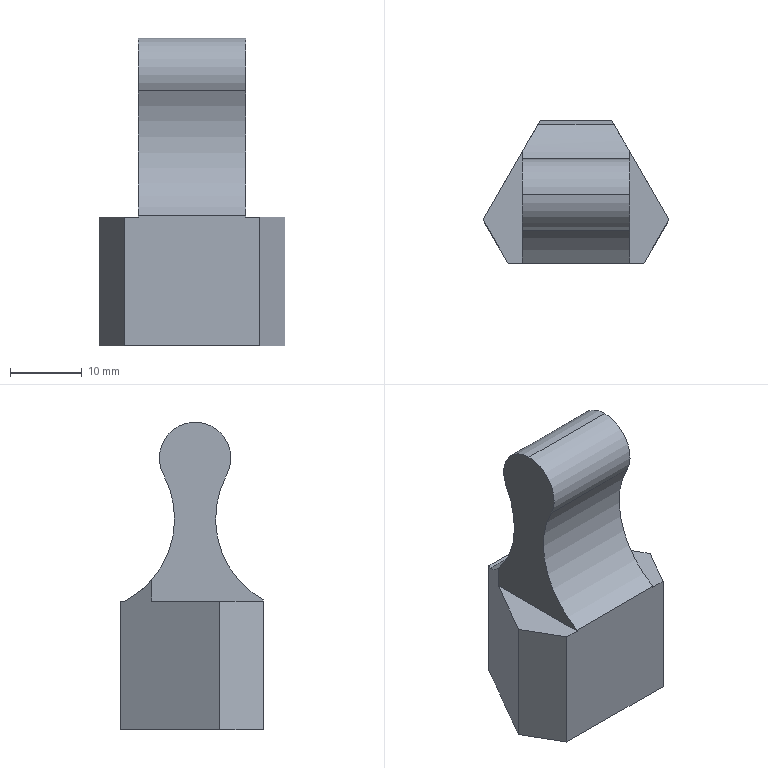Part | STEP file | Seal sleeve 8 | 1 solid | 21 faces | box 26 x 19.919 x 43 mm | volume 9352 mm3 | plane 13 | cylinder 8 | commonest cylinder face diameters 10 x4 2.5 x2 26 x2